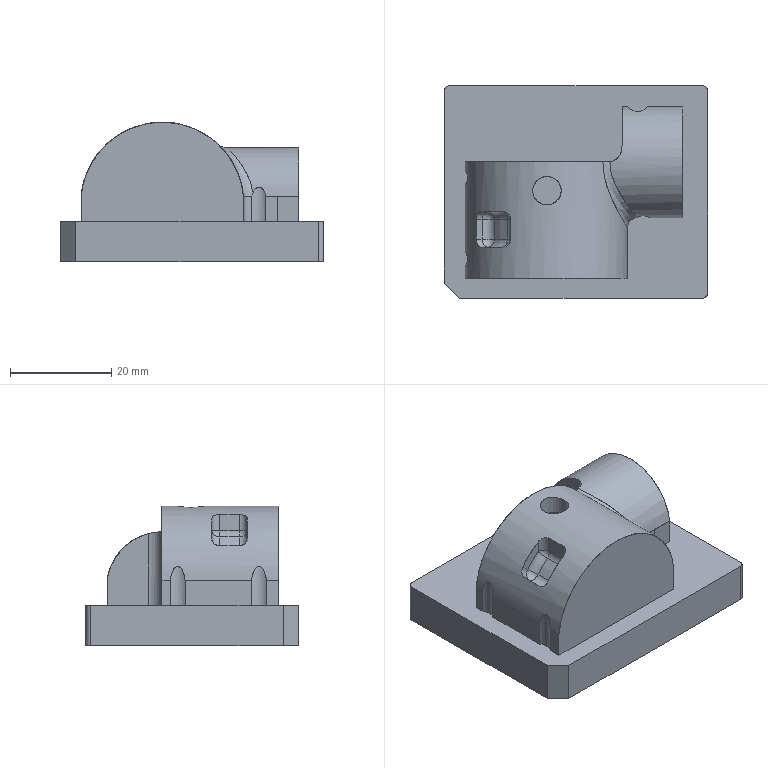NC program | PowerMill | posted with a generic post | part box 52 x 42 x 27.622 mm
Lines 29762 to 30585 of 322299:
N29859 M6
N29860 S18000 M03
N29861 G00 G90 X0.0 Y0.0
N29862 G43 Z9.8022 H28
N29863
N29864 G05 P10000 R4
N29865 X-6.964 Y1.3313
N29866 Z0.893
N29867 G01 Z-0.307 F2400.0
N29868 X-6.9743 Y1.3442 F4000.0
N29869 G03 X-7.183 Y1.3675 I-0.116 J-0.0927
N29870 G01 X-7.2198 Y1.3381
N29871 X-7.5636 Y1.2058
N29872 X-7.9074 Y1.2079
N29873 X-8.2512 Y1.3264
N29874 X-8.3146 Y1.3796
N29875 X-8.5179 Y-0.9378
N29876 X-8.5065 Y-0.9497
N29877 G03 X-8.2965 Y-0.9539 I0.1071 J0.1029
N29878 G01 X-8.1982 Y-0.8595
N29879 X-7.9074 Y-0.7639
N29880 X-7.5636 Y-0.7729
N29881 X-7.2988 Y-0.8595
N29882 X-7.176 Y-0.953
N29883 G00 Z2.853
N29884 G01 X-5.7054 Y0.057 F10000.0
N29885 G00 Z-0.305
N29886 G01 X-5.7933 Y-0.1747 Z-0.3093 F2400.0
N29887 X-6.0535 Y-0.5517 Z-0.3173
N29888 X-6.3963 Y-0.8554 Z-0.3253
N29889 X-6.8019 Y-1.0683 Z-0.3333
N29890 X-6.9156 Y-1.0963 Z-0.3353
N29891 X-7.1956 Y-0.8112 Z-0.3423
N29892 X-7.3706 Y-0.5035 Z-0.3485
N29893 X-7.4812 Y-0.1654 Z-0.3547
N29894 X-7.5219 Y0.1726 Z-0.3606
N29895 X-7.4978 Y0.5107 Z-0.3665
N29896 X-7.4467 Y0.7005 Z-0.37
N29897 X-7.4068 Y0.8484 Z-0.3726
N29898 X-7.1953 Y1.2426 Z-0.3804
N29899 X-6.8571 Y1.5892 Z-0.3889
N29900 X-6.4069 Y1.8633 Z-0.3981
N29901 X-6.1817 Y1.9316 Z-0.4022
N29902 X-6.043 Y1.953 Z-0.4046
N29903 X-5.7933 Y1.5912 Z-0.4123
N29904 X-5.6308 Y1.163 Z-0.4203
N29905 X-5.5756 Y0.7083 Z-0.4283
N29906 X-5.6308 Y0.2536 Z-0.4363
N29907 X-5.7933 Y-0.1747 Z-0.4443
N29908 X-6.0535 Y-0.5517 Z-0.4523
N29909 X-6.3963 Y-0.8554 Z-0.4603
N29910 X-6.8019 Y-1.0683 Z-0.4683
N29911 X-6.9156 Y-1.0963 Z-0.4703
N29912 X-7.1956 Y-0.8112 Z-0.4773
N29913 X-7.3706 Y-0.5035 Z-0.4835
N29914 X-7.4812 Y-0.1654 Z-0.4897
N29915 X-7.5219 Y0.1726 Z-0.4956
N29916 X-7.4978 Y0.5107 Z-0.5015
N29917 X-7.4467 Y0.7005 Z-0.505
N29918 X-7.4756 Y0.7083
N29919 X-6.483 Y0.4188 F4000.0
N29920 X-6.5038 Y0.3226
N29921 X-6.5108 Y0.2245
N29922 G03 X-5.1232 I0.6938 J0.0
N29923 G03 X-6.483 Y0.4188 I-0.6938 J0.0
N29924 G01 X-7.4756 Y0.7083
N29925 X-7.5275 Y0.5157
N29926 X-7.552 Y0.1719
N29927 X-7.5106 Y-0.1719
N29928 X-7.3982 Y-0.5157
N29929 X-7.2198 Y-0.8295
N29930 X-6.876 Y-1.1795
N29931 X-6.5322 Y-1.4005
N29932 X-6.1884 Y-1.5276
N29933 X-5.8446 Y-1.5807
N29934 X-5.4388 Y-1.5526
N29935 X-5.1578 Y-1.4862
N29936 X-5.157 Y-1.4859
N29937 X-4.8132 Y-1.3268
N29938 X-4.4694 Y-1.0663
N29939 X-4.2858 Y-0.8595
N29940 X-4.1256 Y-0.5987
N29941 X-3.9696 Y-0.1719
N29942 X-3.9268 Y0.1719
N29943 X-3.9551 Y0.5157
N29944 X-4.0493 Y0.8595
N29945 X-4.2234 Y1.2033
N29946 X-4.4694 Y1.4997
N29947 X-4.8132 Y1.7601
N29948 X-5.0641 Y1.8909
N29949 X-5.5008 Y2.0005
N29950 X-5.8446 Y2.0141
N29951 X-6.1884 Y1.9609
N29952 X-6.4193 Y1.8909
N29953 X-6.876 Y1.6128
N29954 X-7.2198 Y1.2605
N29955 X-7.4349 Y0.8595
N29956 X-7.4756 Y0.7083
N29957 X-5.7053 Y0.0572 Z-0.4039
N29958 X-5.7933 Y-0.1749 Z-0.4083 F2400.0
N29959 X-6.0535 Y-0.5518 Z-0.4163
N29960 X-6.3963 Y-0.8556 Z-0.4243
N29961 X-6.8019 Y-1.0684 Z-0.4323
N29962 X-6.9155 Y-1.0964 Z-0.4343
N29963 X-7.1956 Y-0.8112 Z-0.4413
N29964 X-7.3706 Y-0.5035 Z-0.4474
N29965 X-7.4811 Y-0.1654 Z-0.4537
N29966 X-7.5219 Y0.1726 Z-0.4596
N29967 X-7.4978 Y0.5107 Z-0.4655
N29968 X-7.4467 Y0.7003 Z-0.4689
N29969 X-7.4068 Y0.8483 Z-0.4716
N29970 X-7.1953 Y1.241 Z-0.4794
N29971 X-6.8571 Y1.5892 Z-0.4879
N29972 X-6.4069 Y1.8633 Z-0.4971
N29973 X-6.1817 Y1.9316 Z-0.5012
N29974 X-6.0431 Y1.953 Z-0.5036
N29975 X-5.7933 Y1.5911 Z-0.5113
N29976 X-5.6309 Y1.1628 Z-0.5193
N29977 X-5.5757 Y0.7081 Z-0.5273
N29978 X-5.6309 Y0.2534 Z-0.5353
N29979 X-5.7933 Y-0.1749 Z-0.5433
N29980 X-6.0535 Y-0.5518 Z-0.5513
N29981 X-6.3963 Y-0.8556 Z-0.5593
N29982 X-6.8019 Y-1.0684 Z-0.5673
N29983 X-6.9155 Y-1.0964 Z-0.5693
N29984 X-7.1956 Y-0.8112 Z-0.5763
N29985 X-7.3706 Y-0.5035 Z-0.5824
N29986 X-7.4811 Y-0.1654 Z-0.5887
N29987 X-7.5219 Y0.1726 Z-0.5946
N29988 X-7.4978 Y0.5107 Z-0.6005
N29989 X-7.4467 Y0.7003 Z-0.6039
N29990 X-7.4757 Y0.7081
N29991 X-6.4841 Y0.4189 F4000.0
N29992 X-6.5048 Y0.3227
N29993 X-6.5118 Y0.2246
N29994 G03 X-5.1241 I0.6939 J0.0
N29995 G03 X-6.4841 Y0.4189 I-0.6938 J0.0
N29996 G01 X-7.4757 Y0.7081
N29997 X-7.5275 Y0.5157
N29998 X-7.552 Y0.1719
N29999 X-7.5105 Y-0.1719
N30000 X-7.3982 Y-0.5157
N30001 X-7.2198 Y-0.8294
N30002 X-6.876 Y-1.1795
N30003 X-6.5322 Y-1.4005
N30004 X-6.1884 Y-1.5276
N30005 X-5.8446 Y-1.5807
N30006 X-5.4385 Y-1.5526
N30007 X-5.1586 Y-1.4864
N30008 X-5.157 Y-1.4859
N30009 X-4.8132 Y-1.3268
N30010 X-4.4694 Y-1.0663
N30011 X-4.2871 Y-0.8595
N30012 X-4.1256 Y-0.5975
N30013 X-3.971 Y-0.1719
N30014 X-3.9288 Y0.1719
N30015 X-3.9563 Y0.5157
N30016 X-4.0501 Y0.8595
N30017 X-4.2249 Y1.2033
N30018 X-4.4694 Y1.4997
N30019 X-4.8132 Y1.7601
N30020 X-5.0641 Y1.8909
N30021 X-5.5008 Y2.0005
N30022 X-5.8446 Y2.0141
N30023 X-6.1884 Y1.9609
N30024 X-6.4193 Y1.8909
N30025 X-6.876 Y1.6128
N30026 X-7.2198 Y1.2589
N30027 X-7.4349 Y0.8595
N30028 X-7.4757 Y0.7081
N30029 X-5.7052 Y0.0574 Z-0.5029
N30030 X-5.7933 Y-0.175 Z-0.5073 F2400.0
N30031 X-6.0535 Y-0.552 Z-0.5153
N30032 X-6.3964 Y-0.8557 Z-0.5233
N30033 X-6.8019 Y-1.0686 Z-0.5312
N30034 X-6.9154 Y-1.0965 Z-0.5333
N30035 X-7.1956 Y-0.8112 Z-0.5403
N30036 X-7.3706 Y-0.5035 Z-0.5464
N30037 X-7.481 Y-0.1654 Z-0.5527
N30038 X-7.5219 Y0.1726 Z-0.5586
N30039 X-7.4978 Y0.5107 Z-0.5645
N30040 X-7.4467 Y0.7001 Z-0.5679
N30041 X-7.4068 Y0.8483 Z-0.5706
N30042 X-7.1953 Y1.2393 Z-0.5784
N30043 X-6.8571 Y1.5892 Z-0.5869
N30044 X-6.4069 Y1.8633 Z-0.5961
N30045 X-6.1817 Y1.9316 Z-0.6002
N30046 X-6.0433 Y1.953 Z-0.6026
N30047 X-5.7933 Y1.5909 Z-0.6103
N30048 X-5.6309 Y1.1626 Z-0.6183
N30049 X-5.5757 Y0.7079 Z-0.6263
N30050 X-5.6309 Y0.2532 Z-0.6343
N30051 X-5.7933 Y-0.175 Z-0.6423
N30052 X-6.0535 Y-0.552 Z-0.6503
N30053 X-6.3964 Y-0.8557 Z-0.6583
N30054 X-6.8019 Y-1.0686 Z-0.6662
N30055 X-6.9154 Y-1.0965 Z-0.6683
N30056 X-7.1956 Y-0.8112 Z-0.6753
N30057 X-7.3706 Y-0.5035 Z-0.6814
N30058 X-7.481 Y-0.1654 Z-0.6876
N30059 X-7.5219 Y0.1726 Z-0.6936
N30060 X-7.4978 Y0.5107 Z-0.6995
N30061 X-7.4467 Y0.7001 Z-0.7029
N30062 X-7.4757 Y0.7079
N30063 X-6.4851 Y0.419 F4000.0
N30064 X-6.5059 Y0.3228
N30065 X-6.5129 Y0.2247
N30066 G03 X-5.1249 I0.694 J0.0
N30067 G03 X-6.4851 Y0.419 I-0.694 J0.0
N30068 G01 X-7.4757 Y0.7079
N30069 X-7.5275 Y0.5157
N30070 X-7.552 Y0.1719
N30071 X-7.5105 Y-0.1719
N30072 X-7.3982 Y-0.5157
N30073 X-7.2198 Y-0.8294
N30074 X-6.876 Y-1.1795
N30075 X-6.5322 Y-1.4005
N30076 X-6.1884 Y-1.5276
N30077 X-5.8446 Y-1.5807
N30078 X-5.4382 Y-1.5526
N30079 X-5.1595 Y-1.4866
N30080 X-5.157 Y-1.4859
N30081 X-4.8132 Y-1.3268
N30082 X-4.4694 Y-1.0663
N30083 X-4.2884 Y-0.8595
N30084 X-4.1256 Y-0.5963
N30085 X-3.9724 Y-0.1719
N30086 X-3.9307 Y0.1719
N30087 X-3.9574 Y0.5157
N30088 X-4.0512 Y0.8595
N30089 X-4.2264 Y1.2033
N30090 X-4.4694 Y1.4997
N30091 X-4.8132 Y1.7601
N30092 X-5.0641 Y1.8909
N30093 X-5.5008 Y2.0005
N30094 X-5.8446 Y2.0141
N30095 X-6.1884 Y1.9609
N30096 X-6.4193 Y1.8909
N30097 X-6.876 Y1.6128
N30098 X-7.2198 Y1.2572
N30099 X-7.4348 Y0.8595
N30100 X-7.4757 Y0.7079
N30101 X-5.7051 Y0.0576 Z-0.6019
N30102 X-5.7934 Y-0.1752 Z-0.6063 F2400.0
N30103 X-6.0536 Y-0.5522 Z-0.6143
N30104 X-6.3964 Y-0.8559 Z-0.6223
N30105 X-6.802 Y-1.0688 Z-0.6302
N30106 X-6.9152 Y-1.0967 Z-0.6323
N30107 X-7.1956 Y-0.8112 Z-0.6393
N30108 X-7.3706 Y-0.5035 Z-0.6454
N30109 X-7.481 Y-0.1654 Z-0.6516
N30110 X-7.5219 Y0.1726 Z-0.6576
N30111 X-7.4978 Y0.5107 Z-0.6635
N30112 X-7.4468 Y0.7 Z-0.6669
N30113 X-7.4068 Y0.8483 Z-0.6696
N30114 X-7.1953 Y1.2376 Z-0.6773
N30115 X-6.8571 Y1.5892 Z-0.6859
N30116 X-6.4069 Y1.8633 Z-0.6951
N30117 X-6.1817 Y1.9316 Z-0.6992
N30118 X-6.0434 Y1.953 Z-0.7016
N30119 X-5.7934 Y1.5907 Z-0.7093
N30120 X-5.6309 Y1.1625 Z-0.7173
N30121 X-5.5757 Y0.7078 Z-0.7253
N30122 X-5.6309 Y0.2531 Z-0.7333
N30123 X-5.7934 Y-0.1752 Z-0.7413
N30124 X-6.0536 Y-0.5522 Z-0.7493
N30125 X-6.3964 Y-0.8559 Z-0.7572
N30126 X-6.802 Y-1.0688 Z-0.7652
N30127 X-6.9152 Y-1.0967 Z-0.7673
N30128 X-7.1956 Y-0.8112 Z-0.7743
N30129 X-7.3706 Y-0.5035 Z-0.7804
N30130 X-7.481 Y-0.1654 Z-0.7866
N30131 X-7.5219 Y0.1726 Z-0.7926
N30132 X-7.4978 Y0.5107 Z-0.7985
N30133 X-7.4468 Y0.7 Z-0.8019
N30134 X-7.4757 Y0.7078
N30135 X-6.4861 Y0.4191 F4000.0
N30136 X-6.5069 Y0.323
N30137 X-6.5139 Y0.2248
N30138 G03 X-5.1257 I0.6941 J0.0
N30139 G03 X-6.4861 Y0.4191 I-0.6941 J0.0
N30140 G01 X-7.4757 Y0.7078
N30141 X-7.5275 Y0.5157
N30142 X-7.552 Y0.1719
N30143 X-7.5105 Y-0.1719
N30144 X-7.3981 Y-0.5157
N30145 X-7.2198 Y-0.8294
N30146 X-6.876 Y-1.1795
N30147 X-6.5322 Y-1.4005
N30148 X-6.1884 Y-1.5276
N30149 X-5.8446 Y-1.5807
N30150 X-5.4378 Y-1.5526
N30151 X-5.1603 Y-1.4869
N30152 X-5.157 Y-1.4859
N30153 X-4.8132 Y-1.3268
N30154 X-4.4694 Y-1.0663
N30155 X-4.2897 Y-0.8595
N30156 X-4.1256 Y-0.595
N30157 X-3.9738 Y-0.1719
N30158 X-3.9327 Y0.1719
N30159 X-3.9585 Y0.5157
N30160 X-4.0524 Y0.8595
N30161 X-4.2275 Y1.2033
N30162 X-4.4694 Y1.4997
N30163 X-4.8132 Y1.7601
N30164 X-5.0641 Y1.8909
N30165 X-5.5008 Y2.0005
N30166 X-5.8446 Y2.0141
N30167 X-6.1884 Y1.9609
N30168 X-6.4193 Y1.8909
N30169 X-6.876 Y1.6128
N30170 X-7.2198 Y1.2555
N30171 X-7.4348 Y0.8595
N30172 X-7.4757 Y0.7078
N30173 X-5.705 Y0.0578 Z-0.7009
N30174 X-5.7934 Y-0.1754 Z-0.7053 F2400.0
N30175 X-6.0536 Y-0.5523 Z-0.7133
N30176 X-6.3964 Y-0.8561 Z-0.7212
N30177 X-6.802 Y-1.0689 Z-0.7292
N30178 X-6.9151 Y-1.0968 Z-0.7313
N30179 X-7.1956 Y-0.8112 Z-0.7383
N30180 X-7.3706 Y-0.5035 Z-0.7444
N30181 X-7.481 Y-0.1654 Z-0.7506
N30182 X-7.5219 Y0.1726 Z-0.7566
N30183 X-7.4978 Y0.5107 Z-0.7625
N30184 X-7.4468 Y0.6998 Z-0.7659
N30185 X-7.4068 Y0.8483 Z-0.7686
N30186 X-7.1954 Y1.236 Z-0.7763
N30187 X-6.857 Y1.5892 Z-0.7848
N30188 X-6.4069 Y1.8633 Z-0.794
N30189 X-6.1817 Y1.9316 Z-0.7982
N30190 X-6.0435 Y1.953 Z-0.8006
N30191 X-5.7934 Y1.5906 Z-0.8083
N30192 X-5.631 Y1.1623 Z-0.8163
N30193 X-5.5758 Y0.7076 Z-0.8243
N30194 X-5.631 Y0.2529 Z-0.8323
N30195 X-5.7934 Y-0.1754 Z-0.8403
N30196 X-6.0536 Y-0.5523 Z-0.8482
N30197 X-6.3964 Y-0.8561 Z-0.8562
N30198 X-6.802 Y-1.0689 Z-0.8642
N30199 X-6.9151 Y-1.0968 Z-0.8663
N30200 X-7.1956 Y-0.8112 Z-0.8733
N30201 X-7.3706 Y-0.5035 Z-0.8794
N30202 X-7.481 Y-0.1654 Z-0.8856
N30203 X-7.5219 Y0.1726 Z-0.8916
N30204 X-7.4978 Y0.5107 Z-0.8975
N30205 X-7.4468 Y0.6998 Z-0.9009
N30206 X-7.4758 Y0.7076
N30207 X-6.4871 Y0.4193 F4000.0
N30208 X-6.5079 Y0.3231
N30209 X-6.5149 Y0.2249
N30210 G03 X-5.1265 I0.6942 J0.0
N30211 G03 X-6.4871 Y0.4193 I-0.6942 J0.0
N30212 G01 X-7.4758 Y0.7076
N30213 X-7.5275 Y0.5157
N30214 X-7.552 Y0.1719
N30215 X-7.5104 Y-0.1719
N30216 X-7.3981 Y-0.5157
N30217 X-7.2198 Y-0.8294
N30218 X-6.876 Y-1.1794
N30219 X-6.5322 Y-1.4005
N30220 X-6.1884 Y-1.5276
N30221 X-5.8446 Y-1.5807
N30222 X-5.4375 Y-1.5525
N30223 X-5.1611 Y-1.4871
N30224 X-5.157 Y-1.4859
N30225 X-4.8132 Y-1.3268
N30226 X-4.4694 Y-1.0663
N30227 X-4.291 Y-0.8595
N30228 X-4.1256 Y-0.5938
N30229 X-3.9753 Y-0.1719
N30230 X-3.9347 Y0.1719
N30231 X-3.9597 Y0.5157
N30232 X-4.0537 Y0.8595
N30233 X-4.2284 Y1.2033
N30234 X-4.4694 Y1.4997
N30235 X-4.8132 Y1.7601
N30236 X-5.0641 Y1.8909
N30237 X-5.5008 Y2.0005
N30238 X-5.8446 Y2.0141
N30239 X-6.1884 Y1.9609
N30240 X-6.4193 Y1.8909
N30241 X-6.876 Y1.6128
N30242 X-7.2198 Y1.2538
N30243 X-7.4348 Y0.8595
N30244 X-7.4758 Y0.7076
N30245 X-5.5428 Y0.1676 Z-0.7999
N30246 X-5.2906 Y-0.1977 Z-0.8076 F2400.0
N30247 X-5.1282 Y-0.626 Z-0.8156
N30248 X-5.073 Y-1.0807 Z-0.8236
N30249 X-5.1159 Y-1.4338 Z-0.8298
N30250 X-5.1677 Y-1.4578 Z-0.8308
N30251 X-5.1698 Y-1.4584 Z-0.8309
N30252 X-5.4417 Y-1.5228 Z-0.8357
N30253 X-5.8433 Y-1.5506 Z-0.8428
N30254 X-6.1808 Y-1.4984 Z-0.8487
N30255 X-6.5187 Y-1.3735 Z-0.855
N30256 X-6.8569 Y-1.156 Z-0.862
N30257 X-6.9516 Y-1.0597 Z-0.8644
N30258 X-7.1956 Y-0.8112 Z-0.8705
N30259 X-7.3705 Y-0.5035 Z-0.8766
N30260 X-7.481 Y-0.1654 Z-0.8829
N30261 X-7.5218 Y0.1726 Z-0.8888
N30262 X-7.4978 Y0.5107 Z-0.8947
N30263 X-7.4337 Y0.7484 Z-0.899
N30264 X-7.202 Y0.8055 Z-0.9032
N30265 X-6.744 Z-0.9112
N30266 X-6.2992 Y0.6959 Z-0.9192
N30267 X-5.8937 Y0.483 Z-0.9271
N30268 X-5.5508 Y0.1793 Z-0.9351
N30269 X-5.2906 Y-0.1977 Z-0.9431
N30270 X-5.1282 Y-0.626 Z-0.9511
N30271 X-5.073 Y-1.0807 Z-0.9591
N30272 X-5.1159 Y-1.4338 Z-0.9653
N30273 X-5.1677 Y-1.4578 Z-0.9663
N30274 X-5.1698 Y-1.4584 Z-0.9664
N30275 X-5.4417 Y-1.5228 Z-0.9712
N30276 X-5.8433 Y-1.5506 Z-0.9783
N30277 X-6.1808 Y-1.4984 Z-0.9842
N30278 X-6.5187 Y-1.3735 Z-0.9905
N30279 X-6.8569 Y-1.156 Z-0.9975
N30280 X-6.9516 Y-1.0597 Z-0.9999
N30281 X-6.973 Y-1.0807
N30282 X-6.1624 Y-0.2239 F4000.0
N30283 G03 X-5.5515 Y-0.3593 I0.4185 J0.4423
N30284 G01 X-5.5485 Y-0.3583
N30285 G03 X-5.1639 Y0.4135 I-0.1925 J0.5777
N30286 G03 X-5.9367 Y0.7959 I-0.5771 J-0.1941
N30287 G01 X-5.9397 Y0.7949
N30288 G03 X-6.1624 Y-0.2239 I0.1958 J-0.5765
N30289 G01 X-6.973 Y-1.0807
N30290 X-6.876 Y-1.1794
N30291 X-6.5322 Y-1.4005
N30292 X-6.1884 Y-1.5276
N30293 X-5.8446 Y-1.5807
N30294 X-5.4372 Y-1.5525
N30295 X-5.162 Y-1.4874
N30296 X-5.157 Y-1.4859
N30297 X-4.8132 Y-1.3268
N30298 X-4.4694 Y-1.0663
N30299 X-4.2923 Y-0.8595
N30300 X-4.1256 Y-0.5926
N30301 X-3.9767 Y-0.1719
N30302 X-3.942 Y0.2733
N30303 X-3.9521 Y0.4124
N30304 X-4.0548 Y0.8595
N30305 X-4.2288 Y1.2033
N30306 X-4.4694 Y1.4997
N30307 X-4.8132 Y1.7601
N30308 X-5.0641 Y1.8909
N30309 X-5.5008 Y2.0005
N30310 X-5.8446 Y2.0141
N30311 X-6.1884 Y1.9609
N30312 X-6.4193 Y1.8909
N30313 X-6.876 Y1.6128
N30314 X-7.2198 Y1.2523
N30315 X-7.4348 Y0.8595
N30316 X-7.5275 Y0.5157
N30317 X-7.552 Y0.1719
N30318 X-7.5104 Y-0.1719
N30319 X-7.3981 Y-0.5157
N30320 X-7.2198 Y-0.8294
N30321 X-6.973 Y-1.0807
N30322 X-5.7048 Y0.058 Z-0.8989
N30323 X-5.7935 Y-0.1758 Z-0.9032 F2400.0
N30324 X-6.0537 Y-0.5528 Z-0.9112
N30325 X-6.3965 Y-0.8565 Z-0.9192
N30326 X-6.8021 Y-1.0694 Z-0.9272
N30327 X-6.9148 Y-1.0971 Z-0.9293
N30328 X-7.1956 Y-0.8112 Z-0.9362
N30329 X-7.3705 Y-0.5035 Z-0.9424
N30330 X-7.481 Y-0.1654 Z-0.9486
N30331 X-7.5218 Y0.1726 Z-0.9546
N30332 X-7.4977 Y0.5107 Z-0.9605
N30333 X-7.4469 Y0.6993 Z-0.9639
N30334 X-7.4068 Y0.8482 Z-0.9666
N30335 X-7.1954 Y1.2337 Z-0.9743
N30336 X-6.857 Y1.5892 Z-0.9828
N30337 X-6.4069 Y1.8633 Z-0.992
N30338 X-6.1817 Y1.9316 Z-0.9961
N30339 X-6.0439 Y1.9529 Z-0.9986
N30340 X-5.7935 Y1.5901 Z-1.0063
N30341 X-5.6311 Y1.1618 Z-1.0142
N30342 X-5.5759 Y0.7071 Z-1.0222
N30343 X-5.6311 Y0.2524 Z-1.0302
N30344 X-5.7935 Y-0.1758 Z-1.0382
N30345 X-6.0537 Y-0.5528 Z-1.0462
N30346 X-6.3965 Y-0.8565 Z-1.0542
N30347 X-6.8021 Y-1.0694 Z-1.0622
N30348 X-6.9148 Y-1.0971 Z-1.0642
N30349 X-7.1956 Y-0.8112 Z-1.0712
N30350 X-7.3705 Y-0.5035 Z-1.0774
N30351 X-7.481 Y-0.1654 Z-1.0836
N30352 X-7.5218 Y0.1726 Z-1.0896
N30353 X-7.4977 Y0.5107 Z-1.0955
N30354 X-7.4469 Y0.6993 Z-1.0989
N30355 X-7.4759 Y0.7071
N30356 X-6.49 Y0.4196 F4000.0
N30357 X-6.5108 Y0.3234
N30358 X-6.5178 Y0.2251
N30359 G03 X-5.1288 I0.6945 J0.0
N30360 G03 X-6.49 Y0.4196 I-0.6945 J0.0
N30361 G01 X-7.4759 Y0.7071
N30362 X-7.5275 Y0.5157
N30363 X-7.552 Y0.1719
N30364 X-7.5104 Y-0.1719
N30365 X-7.3981 Y-0.5157
N30366 X-7.2198 Y-0.8294
N30367 X-6.876 Y-1.1794
N30368 X-6.5322 Y-1.4005
N30369 X-6.1884 Y-1.5276
N30370 X-5.8446 Y-1.5807
N30371 X-5.4369 Y-1.5525
N30372 X-5.1628 Y-1.4876
N30373 X-5.157 Y-1.4859
N30374 X-4.8132 Y-1.3268
N30375 X-4.4694 Y-1.0663
N30376 X-4.2935 Y-0.8595
N30377 X-4.1256 Y-0.5899
N30378 X-3.9781 Y-0.1719
N30379 X-3.9738 Y-0.1363
N30380 X-3.9433 Y0.2563
N30381 X-3.9556 Y0.428
N30382 X-4.0499 Y0.8388
N30383 X-4.0556 Y0.8595
N30384 X-4.2292 Y1.2033
N30385 X-4.4694 Y1.4997
N30386 X-4.8132 Y1.7601
N30387 X-5.0641 Y1.8909
N30388 X-5.5008 Y2.0005
N30389 X-5.8446 Y2.0141
N30390 X-6.1884 Y1.9609
N30391 X-6.4193 Y1.8909
N30392 X-6.876 Y1.6128
N30393 X-7.2198 Y1.2516
N30394 X-7.4348 Y0.8595
N30395 X-7.4759 Y0.7071
N30396 X-5.562 Y0.3125 Z-0.9979
N30397 X-5.5136 Z-0.9987 F2400.0
N30398 X-5.0688 Y0.2029 Z-1.0067
N30399 X-4.6633 Y-0.01 Z-1.0147
N30400 X-4.3204 Y-0.3137 Z-1.0227
N30401 X-4.1487 Y-0.5625 Z-1.028
N30402 X-4.1528 Y-0.574 Z-1.0282
N30403 X-4.3192 Y-0.8418 Z-1.0337
N30404 X-4.4902 Y-1.0444 Z-1.0383
N30405 X-4.8287 Y-1.3009 Z-1.0457
N30406 X-5.1677 Y-1.4578 Z-1.0522
N30407 X-5.1714 Y-1.4589 Z-1.0523
N30408 X-5.4411 Y-1.5227 Z-1.0571
N30409 X-5.7447 Y-1.5437 Z-1.0625
N30410 X-5.8433 Y-1.5506 Z-1.0642
N30411 X-6.1808 Y-1.4984 Z-1.0701
N30412 X-6.5187 Y-1.3735 Z-1.0764
N30413 X-6.8569 Y-1.156 Z-1.0834
N30414 X-7.1956 Y-0.8111 Z-1.0919
N30415 X-7.3368 Y-0.5629 Z-1.0969
N30416 X-7.1648 Y-0.3137 Z-1.1022
N30417 X-6.8219 Y-0.01 Z-1.1101
N30418 X-6.4163 Y0.2029 Z-1.1181
N30419 X-5.9716 Y0.3125 Z-1.1261
N30420 X-5.5136 Z-1.1341
N30421 X-5.0688 Y0.2029 Z-1.1421
N30422 X-4.6633 Y-0.01 Z-1.1501
N30423 X-4.3204 Y-0.3137 Z-1.1581
N30424 X-4.1487 Y-0.5625 Z-1.1634
N30425 X-4.1528 Y-0.574 Z-1.1636
N30426 X-4.3192 Y-0.8418 Z-1.1691
N30427 X-4.4902 Y-1.0444 Z-1.1737
N30428 X-4.8287 Y-1.3009 Z-1.1811
N30429 X-5.1677 Y-1.4578 Z-1.1877
N30430 X-5.1714 Y-1.4589
N30431 X-5.4411 Y-1.5227 Z-1.1926
N30432 X-5.7447 Y-1.5437 Z-1.1979
N30433 X-5.7426 Y-1.5736
N30434 Y-0.5582 F4000.0
N30435 G03 X-5.0505 Y0.1339 I0.0 J0.6921
N30436 G03 X-6.4347 I-0.6921 J0.0
N30437 G03 X-5.7426 Y-0.5582 I0.6921 J0.0
N30438 G01 Y-1.5736
N30439 X-5.4366 Y-1.5525
N30440 X-5.1636 Y-1.4879
N30441 X-5.157 Y-1.4859
N30442 X-4.8132 Y-1.3268
N30443 X-4.4694 Y-1.0663
N30444 X-4.2948 Y-0.8595
N30445 X-4.1256 Y-0.5871
N30446 X-3.9795 Y-0.1719
N30447 X-3.9714 Y-0.105
N30448 X-3.9436 Y0.252
N30449 X-3.9567 Y0.433
N30450 X-4.0457 Y0.8205
N30451 X-4.0563 Y0.8595
N30452 X-4.2293 Y1.2033
N30453 X-4.4694 Y1.4997
N30454 X-4.8132 Y1.7601
N30455 X-5.0641 Y1.8909
N30456 X-5.5008 Y2.0005
N30457 X-5.8446 Y2.0141
N30458 X-6.1884 Y1.9609
N30459 X-6.4193 Y1.8909
N30460 X-6.876 Y1.6128
N30461 X-7.2284 Y1.236
N30462 X-7.4334 Y0.862
N30463 X-7.4347 Y0.8595
N30464 X-7.5275 Y0.5157
N30465 X-7.552 Y0.1719
N30466 X-7.5104 Y-0.1719
N30467 X-7.3981 Y-0.5157
N30468 X-7.2198 Y-0.8294
N30469 X-6.876 Y-1.1794
N30470 X-6.5322 Y-1.4005
N30471 X-6.1884 Y-1.5276
N30472 X-5.8446 Y-1.5807
N30473 X-5.7426 Y-1.5736
N30474 X-5.5637 Y0.3125 Z-1.0969
N30475 X-5.5136 Z-1.0977 F2400.0
N30476 X-5.0689 Y0.2029 Z-1.1057
N30477 X-4.6633 Y-0.01 Z-1.1137
N30478 X-4.3205 Y-0.3137 Z-1.1217
N30479 X-4.1494 Y-0.5616 Z-1.127
N30480 X-4.1528 Y-0.5712 Z-1.1271
N30481 X-4.3203 Y-0.8419 Z-1.1327
N30482 X-4.4902 Y-1.0445 Z-1.1373
N30483 X-4.8287 Y-1.3009 Z-1.1447
N30484 X-5.1677 Y-1.4578 Z-1.1512
N30485 X-5.1723 Y-1.4592 Z-1.1513
N30486 X-5.4408 Y-1.5227 Z-1.1561
N30487 X-5.7447 Y-1.5437 Z-1.1615
N30488 X-5.8433 Y-1.5505 Z-1.1632
N30489 X-6.1808 Y-1.4984 Z-1.1691
N30490 X-6.5187 Y-1.3734 Z-1.1754
N30491 X-6.8569 Y-1.156 Z-1.1825
N30492 X-7.1956 Y-0.8111 Z-1.1909
N30493 X-7.3368 Y-0.5628 Z-1.1959
N30494 X-7.1648 Y-0.3137 Z-1.2012
N30495 X-6.822 Y-0.01 Z-1.2091
N30496 X-6.4164 Y0.2029 Z-1.2171
N30497 X-5.9717 Y0.3125 Z-1.2251
N30498 X-5.5136 Z-1.2331
N30499 X-5.0689 Y0.2029 Z-1.2411
N30500 X-4.6633 Y-0.01 Z-1.2491
N30501 X-4.3205 Y-0.3137 Z-1.2571
N30502 X-4.1494 Y-0.5616 Z-1.2624
N30503 X-4.1528 Y-0.5712 Z-1.2625
N30504 X-4.3203 Y-0.8419 Z-1.2681
N30505 X-4.4902 Y-1.0445 Z-1.2727
N30506 X-4.8287 Y-1.3009 Z-1.2801
N30507 X-5.1677 Y-1.4578 Z-1.2866
N30508 X-5.1723 Y-1.4592 Z-1.2867
N30509 X-5.4408 Y-1.5227 Z-1.2915
N30510 X-5.7447 Y-1.5437 Z-1.2969
N30511 X-5.7427 Y-1.5737
N30512 Y-0.5579 F4000.0
N30513 G03 X-5.0507 Y0.1341 I0.0 J0.692
N30514 G03 X-6.4347 I-0.692 J0.0
N30515 G03 X-5.7427 Y-0.5579 I0.692 J0.0
N30516 G01 Y-1.5737
N30517 X-5.4363 Y-1.5524
N30518 X-5.1644 Y-1.4881
N30519 X-5.157 Y-1.4859
N30520 X-4.8132 Y-1.3268
N30521 X-4.4694 Y-1.0663
N30522 X-4.296 Y-0.8595
N30523 X-4.1256 Y-0.5842
N30524 X-3.9797 Y-0.1719
N30525 X-3.9707 Y-0.0975
N30526 X-3.9438 Y0.2482
N30527 X-3.9575 Y0.4366
N30528 X-4.0431 Y0.8095
N30529 X-4.0567 Y0.8595
N30530 X-4.2293 Y1.2033
N30531 X-4.4694 Y1.4996
N30532 X-4.8132 Y1.7601
N30533 X-5.0641 Y1.8909
N30534 X-5.5008 Y2.0005
N30535 X-5.8446 Y2.0141
N30536 X-6.1884 Y1.9609
N30537 X-6.4193 Y1.8909
N30538 X-6.876 Y1.6128
N30539 X-7.2285 Y1.2358
N30540 X-7.4302 Y0.8682
N30541 X-7.4346 Y0.8595
N30542 X-7.5274 Y0.5157
N30543 X-7.552 Y0.1719
N30544 X-7.5103 Y-0.1719
N30545 X-7.398 Y-0.5157
N30546 X-7.2198 Y-0.8294
N30547 X-6.876 Y-1.1794
N30548 X-6.5322 Y-1.4005
N30549 X-6.1884 Y-1.5276
N30550 X-5.8446 Y-1.5807
N30551 X-5.7427 Y-1.5737
N30552 X-5.5654 Y0.3125 Z-1.1958
N30553 X-5.5137 Z-1.1967 F2400.0
N30554 X-5.0689 Y0.2029 Z-1.2047
N30555 X-4.6634 Y-0.01 Z-1.2127
N30556 X-4.3205 Y-0.3137 Z-1.2207
N30557 X-4.1501 Y-0.5607 Z-1.226
N30558 X-4.1528 Y-0.5683 Z-1.2261
N30559 X-4.3212 Y-0.8419 Z-1.2317
N30560 X-4.4902 Y-1.0445 Z-1.2363
N30561 X-4.8287 Y-1.3009 Z-1.2437
N30562 X-5.1677 Y-1.4578 Z-1.2502
N30563 X-5.1731 Y-1.4594 Z-1.2503
N30564 X-5.4405 Y-1.5227 Z-1.2551
N30565 X-5.7448 Y-1.5437 Z-1.2605
N30566 X-5.8433 Y-1.5505 Z-1.2622
N30567 X-6.1808 Y-1.4984 Z-1.2681
N30568 X-6.5187 Y-1.3734 Z-1.2744
N30569 X-6.8569 Y-1.156 Z-1.2814
N30570 X-7.1956 Y-0.8111 Z-1.2899
N30571 X-7.3367 Y-0.5627 Z-1.2949
N30572 X-7.1649 Y-0.3137 Z-1.3001
N30573 X-6.822 Y-0.01 Z-1.3081
N30574 X-6.4164 Y0.2029 Z-1.3161
N30575 X-5.9717 Y0.3125 Z-1.3241
N30576 X-5.5137 Z-1.3321
N30577 X-5.0689 Y0.2029 Z-1.3401
N30578 X-4.6634 Y-0.01 Z-1.3481
N30579 X-4.3205 Y-0.3137 Z-1.3561
N30580 X-4.1501 Y-0.5607 Z-1.3613
N30581 X-4.1528 Y-0.5683 Z-1.3615
N30582 X-4.3212 Y-0.8419 Z-1.3671
N30583 X-4.4902 Y-1.0445 Z-1.3717
N30584 X-4.8287 Y-1.3009 Z-1.3791
N30585 X-5.1677 Y-1.4578 Z-1.3856
N30586 X-5.1731 Y-1.4594 Z-1.3857
N30587 X-5.4405 Y-1.5227 Z-1.3905
N30588 X-5.7448 Y-1.5437 Z-1.3958
N30589 X-5.7427 Y-1.5736
N30590 Y-0.5578 F4000.0
N30591 G03 X-5.0507 Y0.1341 I0.0 J0.6919
N30592 G03 X-6.4347 I-0.692 J0.0
N30593 G03 X-5.7427 Y-0.5578 I0.692 J0.0
N30594 G01 Y-1.5736
N30595 X-5.436 Y-1.5524
N30596 X-5.1653 Y-1.4884
N30597 X-5.157 Y-1.4859
N30598 X-4.8132 Y-1.3268
N30599 X-4.4694 Y-1.0663
N30600 X-4.2968 Y-0.8595
N30601 X-4.1256 Y-0.5814
N30602 X-3.9797 Y-0.1719
N30603 X-3.9705 Y-0.0951
N30604 X-3.9439 Y0.2464
N30605 X-3.9579 Y0.4383
N30606 X-4.0422 Y0.8058
N30607 X-4.0568 Y0.8595
N30608 X-4.2293 Y1.2033
N30609 X-4.4694 Y1.4996
N30610 X-4.8132 Y1.7601
N30611 X-5.0641 Y1.8909
N30612 X-5.5008 Y2.0005
N30613 X-5.8446 Y2.0141
N30614 X-6.1884 Y1.9609
N30615 X-6.4193 Y1.8909
N30616 X-6.876 Y1.6128
N30617 X-7.2287 Y1.2356
N30618 X-7.4269 Y0.8741
N30619 X-7.4344 Y0.8595
N30620 X-7.5274 Y0.5157
N30621 X-7.552 Y0.1719
N30622 X-7.5103 Y-0.1719
N30623 X-7.3979 Y-0.5157
N30624 X-7.2198 Y-0.8294
N30625 X-6.876 Y-1.1794
N30626 X-6.5322 Y-1.4004
N30627 X-6.1884 Y-1.5276
N30628 X-5.8446 Y-1.5807
N30629 X-5.7427 Y-1.5736
N30630 X-5.567 Y0.3125 Z-1.2948
N30631 X-5.5136 Z-1.2958 F2400.0
N30632 X-5.0689 Y0.2029 Z-1.3038
N30633 X-4.6633 Y-0.01 Z-1.3117
N30634 X-4.3205 Y-0.3137 Z-1.3197
N30635 X-4.1507 Y-0.5598 Z-1.325
N30636 X-4.1528 Y-0.5657 Z-1.3251
N30637 X-4.3218 Y-0.842 Z-1.3307
N30638 X-4.4902 Y-1.0445 Z-1.3353
N30639 X-4.8287 Y-1.3009 Z-1.3427
N30640 X-5.1677 Y-1.4578 Z-1.3492
N30641 X-5.1739 Y-1.4596 Z-1.3494
N30642 X-5.4402 Y-1.5226 Z-1.3541
N30643 X-5.7447 Y-1.5437 Z-1.3595
N30644 X-5.8433 Y-1.5505 Z-1.3612
N30645 X-6.1808 Y-1.4984 Z-1.3671
N30646 X-6.5187 Y-1.3734 Z-1.3734
N30647 X-6.8569 Y-1.156 Z-1.3805
N30648 X-7.1956 Y-0.8111 Z-1.3889
N30649 X-7.3366 Y-0.5626 Z-1.3939
N30650 X-7.1648 Y-0.3137 Z-1.3992
N30651 X-6.822 Y-0.01 Z-1.4071
N30652 X-6.4164 Y0.2029 Z-1.4151
N30653 X-5.9717 Y0.3125 Z-1.4231
N30654 X-5.5136 Z-1.4311
N30655 X-5.0689 Y0.2029 Z-1.4391
N30656 X-4.6633 Y-0.01 Z-1.4471
N30657 X-4.3205 Y-0.3137 Z-1.4551
N30658 X-4.1507 Y-0.5598 Z-1.4603
N30659 X-4.1528 Y-0.5657 Z-1.4604
N30660 X-4.3218 Y-0.842 Z-1.4661
N30661 X-4.4902 Y-1.0445 Z-1.4707
N30662 X-4.8287 Y-1.3009 Z-1.4781
N30663 X-5.1677 Y-1.4578 Z-1.4846
N30664 X-5.1739 Y-1.4596 Z-1.4847
N30665 X-5.4402 Y-1.5226 Z-1.4895
N30666 X-5.7447 Y-1.5437 Z-1.4948
N30667 X-5.7427 Y-1.5736
N30668 Y-0.5579 F4000.0
N30669 G03 X-5.0507 Y0.1341 I0.0 J0.692
N30670 G03 X-6.4347 I-0.692 J0.0
N30671 G03 X-5.7427 Y-0.5579 I0.692 J0.0
N30672 G01 Y-1.5736
N30673 X-5.4357 Y-1.5524
N30674 X-5.1661 Y-1.4886
N30675 X-5.157 Y-1.4859
N30676 X-4.8132 Y-1.3268
N30677 X-4.4694 Y-1.0663
N30678 X-4.2974 Y-0.8595
N30679 X-4.1256 Y-0.5787
N30680 X-3.9797 Y-0.1719
N30681 X-3.9703 Y-0.0938
N30682 X-3.9439 Y0.2461